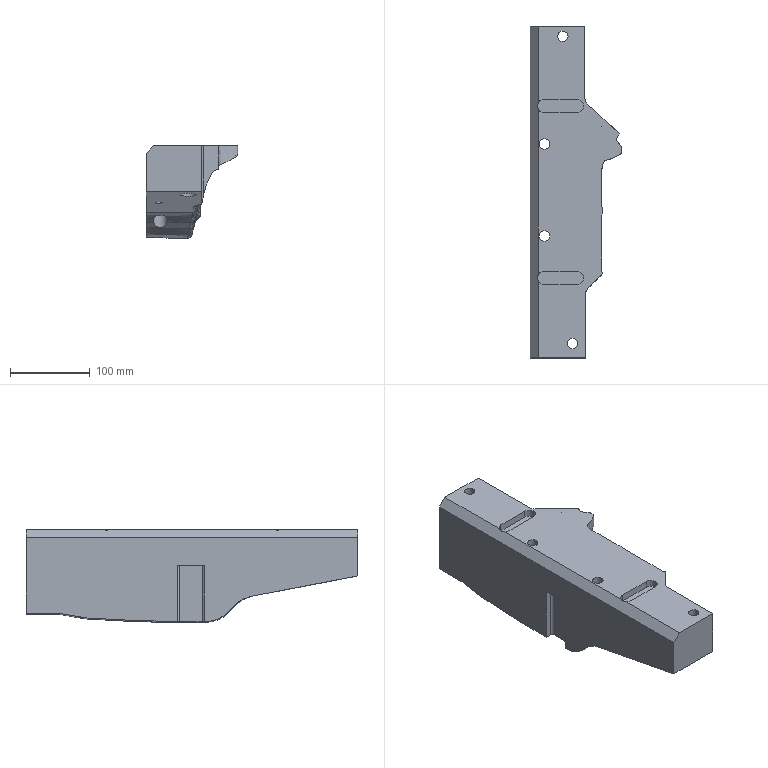Part | NX | features solid 2 | 1 solid | 134 faces | box 115 x 415 x 116.546 mm | volume 2729146 mm3 | spline 66 | plane 34 | cylinder 32 | cone 2 | commonest cylinder face diameters 29 x6 13 x4 16 x4 18.008 x3 105 x3 6 x2